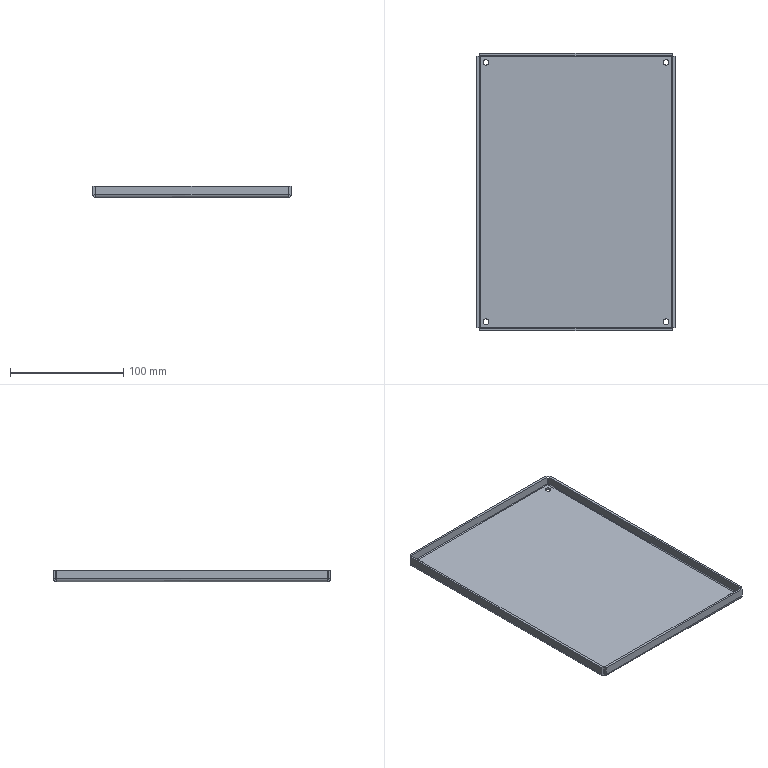Part | STEP file | Ctrl board 11 | 1 solid | 46 faces | box 175 x 245 x 10 mm | volume 97407 mm3 | plane 22 | cylinder 16 | spline 8 | commonest cylinder face diameters 5 x8 1.473 x4 5.473 x4